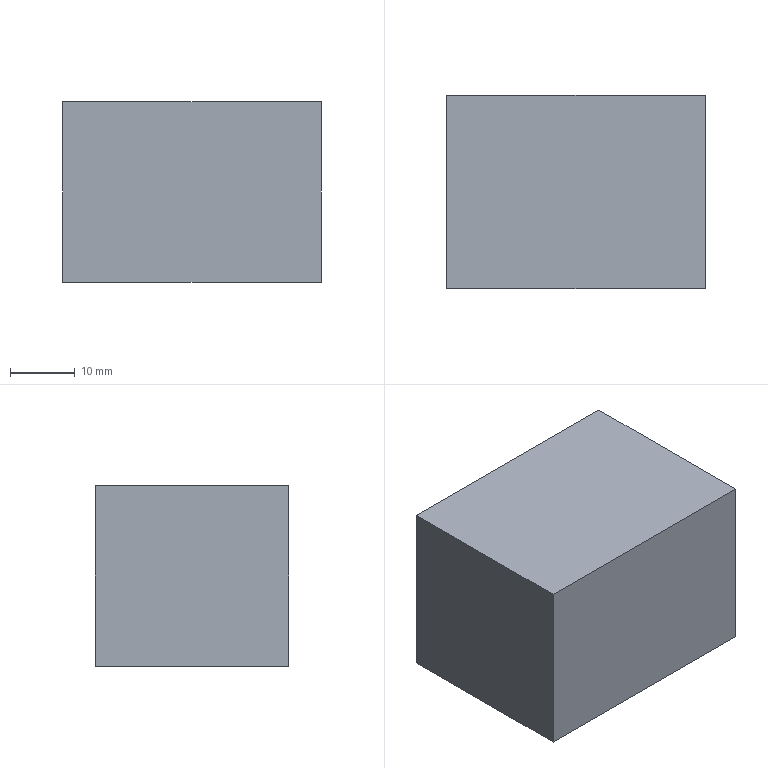Part | NX | features solid 2 | 1 solid | 6 faces | box 40 x 30 x 28 mm | volume 33600 mm3 | plane 6
STEP:
#1=CARTESIAN_POINT('',(-212.,-170.,23.));
#2=VERTEX_POINT('',#1);
#3=CARTESIAN_POINT('',(-252.,-170.,23.));
#4=VERTEX_POINT('',#3);
#5=CARTESIAN_POINT('',(-212.,-170.,23.));
#6=DIRECTION('',(-1.,0.,0.));
#7=VECTOR('',#6,1000.);
#8=LINE('',#5,#7);
#9=EDGE_CURVE('',#2,#4,#8,.T.);
#10=ORIENTED_EDGE('',*,*,#9,.F.);
#11=CARTESIAN_POINT('',(-212.,-140.,23.));
#12=VERTEX_POINT('',#11);
#13=CARTESIAN_POINT('',(-212.,-140.,23.));
#14=DIRECTION('',(0.,-1.,0.));
#15=VECTOR('',#14,1000.);
#16=LINE('',#13,#15);
#17=EDGE_CURVE('',#12,#2,#16,.T.);
#18=ORIENTED_EDGE('',*,*,#17,.F.);
#19=CARTESIAN_POINT('',(-252.,-140.,23.));
#20=VERTEX_POINT('',#19);
#21=CARTESIAN_POINT('',(-212.,-140.,23.));
#22=DIRECTION('',(1.,0.,0.));
#23=VECTOR('',#22,1000.);
#24=LINE('',#21,#23);
#25=EDGE_CURVE('',#12,#20,#24,.F.);
#26=ORIENTED_EDGE('',*,*,#25,.T.);
#27=CARTESIAN_POINT('',(-252.,-140.,23.));
#28=DIRECTION('',(0.,-1.,0.));
#29=VECTOR('',#28,1000.);
#30=LINE('',#27,#29);
#31=EDGE_CURVE('',#20,#4,#30,.T.);
#32=ORIENTED_EDGE('',*,*,#31,.T.);
#33=EDGE_LOOP('',(#10,#18,#26,#32));
#34=FACE_BOUND('',#33,.T.);
#35=CARTESIAN_POINT('',(-212.,-140.,23.));
#36=DIRECTION('',(0.,0.,1.));
#37=DIRECTION('',(0.,-1.,0.));
#38=AXIS2_PLACEMENT_3D('',#35,#36,#37);
#39=PLANE('',#38);
#40=ADVANCED_FACE('',(#34),#39,.T.);
#41=ORIENTED_EDGE('',*,*,#25,.F.);
#42=CARTESIAN_POINT('',(-212.,-140.,-5.));
#43=VERTEX_POINT('',#42);
#44=CARTESIAN_POINT('',(-212.,-140.,85.));
#45=DIRECTION('',(0.,0.,-1.));
#46=VECTOR('',#45,1000.);
#47=LINE('',#44,#46);
#48=EDGE_CURVE('',#12,#43,#47,.T.);
#49=ORIENTED_EDGE('',*,*,#48,.T.);
#50=CARTESIAN_POINT('',(-252.,-140.,-5.));
#51=VERTEX_POINT('',#50);
#52=CARTESIAN_POINT('',(-212.,-140.,-5.));
#53=DIRECTION('',(1.,0.,0.));
#54=VECTOR('',#53,1000.);
#55=LINE('',#52,#54);
#56=EDGE_CURVE('',#43,#51,#55,.F.);
#57=ORIENTED_EDGE('',*,*,#56,.T.);
#58=CARTESIAN_POINT('',(-252.,-140.,85.));
#59=DIRECTION('',(0.,0.,-1.));
#60=VECTOR('',#59,1000.);
#61=LINE('',#58,#60);
#62=EDGE_CURVE('',#20,#51,#61,.T.);
#63=ORIENTED_EDGE('',*,*,#62,.F.);
#64=EDGE_LOOP('',(#41,#49,#57,#63));
#65=FACE_BOUND('',#64,.T.);
#66=CARTESIAN_POINT('',(-212.,-140.,85.));
#67=DIRECTION('',(0.,-1.,0.));
#68=DIRECTION('',(0.,0.,-1.));
#69=AXIS2_PLACEMENT_3D('',#66,#67,#68);
#70=PLANE('',#69);
#71=ADVANCED_FACE('',(#65),#70,.F.);
#72=ORIENTED_EDGE('',*,*,#56,.F.);
#73=CARTESIAN_POINT('',(-212.,-170.,-5.));
#74=VERTEX_POINT('',#73);
#75=CARTESIAN_POINT('',(-212.,-140.,-5.));
#76=DIRECTION('',(0.,-1.,0.));
#77=VECTOR('',#76,1000.);
#78=LINE('',#75,#77);
#79=EDGE_CURVE('',#43,#74,#78,.T.);
#80=ORIENTED_EDGE('',*,*,#79,.T.);
#81=CARTESIAN_POINT('',(-252.,-170.,-5.));
#82=VERTEX_POINT('',#81);
#83=CARTESIAN_POINT('',(-374.173,-170.,-5.));
#84=DIRECTION('',(-1.,0.,0.));
#85=VECTOR('',#84,1000.);
#86=LINE('',#83,#85);
#87=EDGE_CURVE('',#74,#82,#86,.T.);
#88=ORIENTED_EDGE('',*,*,#87,.T.);
#89=CARTESIAN_POINT('',(-252.,-140.,-5.));
#90=DIRECTION('',(0.,-1.,0.));
#91=VECTOR('',#90,1000.);
#92=LINE('',#89,#91);
#93=EDGE_CURVE('',#51,#82,#92,.T.);
#94=ORIENTED_EDGE('',*,*,#93,.F.);
#95=EDGE_LOOP('',(#72,#80,#88,#94));
#96=FACE_BOUND('',#95,.T.);
#97=CARTESIAN_POINT('',(-374.173,-140.,-5.));
#98=DIRECTION('',(0.,0.,-1.));
#99=DIRECTION('',(1.,0.,0.));
#100=AXIS2_PLACEMENT_3D('',#97,#98,#99);
#101=PLANE('',#100);
#102=ADVANCED_FACE('',(#96),#101,.T.);
#103=ORIENTED_EDGE('',*,*,#93,.T.);
#104=CARTESIAN_POINT('',(-252.,-170.,85.));
#105=DIRECTION('',(0.,0.,-1.));
#106=VECTOR('',#105,1000.);
#107=LINE('',#104,#106);
#108=EDGE_CURVE('',#4,#82,#107,.T.);
#109=ORIENTED_EDGE('',*,*,#108,.F.);
#110=ORIENTED_EDGE('',*,*,#31,.F.);
#111=ORIENTED_EDGE('',*,*,#62,.T.);
#112=EDGE_LOOP('',(#103,#109,#110,#111));
#113=FACE_BOUND('',#112,.T.);
#114=CARTESIAN_POINT('',(-252.,-140.,85.));
#115=DIRECTION('',(1.,0.,0.));
#116=DIRECTION('',(0.,0.,-1.));
#117=AXIS2_PLACEMENT_3D('',#114,#115,#116);
#118=PLANE('',#117);
#119=ADVANCED_FACE('',(#113),#118,.F.);
#120=CARTESIAN_POINT('',(-212.,-170.,85.));
#121=DIRECTION('',(0.,0.,-1.));
#122=VECTOR('',#121,1000.);
#123=LINE('',#120,#122);
#124=EDGE_CURVE('',#2,#74,#123,.T.);
#125=ORIENTED_EDGE('',*,*,#124,.F.);
#126=ORIENTED_EDGE('',*,*,#9,.T.);
#127=ORIENTED_EDGE('',*,*,#108,.T.);
#128=ORIENTED_EDGE('',*,*,#87,.F.);
#129=EDGE_LOOP('',(#125,#126,#127,#128));
#130=FACE_BOUND('',#129,.T.);
#131=CARTESIAN_POINT('',(-212.,-170.,85.));
#132=DIRECTION('',(0.,-1.,0.));
#133=DIRECTION('',(0.,0.,-1.));
#134=AXIS2_PLACEMENT_3D('',#131,#132,#133);
#135=PLANE('',#134);
#136=ADVANCED_FACE('',(#130),#135,.T.);
#137=ORIENTED_EDGE('',*,*,#79,.F.);
#138=ORIENTED_EDGE('',*,*,#48,.F.);
#139=ORIENTED_EDGE('',*,*,#17,.T.);
#140=ORIENTED_EDGE('',*,*,#124,.T.);
#141=EDGE_LOOP('',(#137,#138,#139,#140));
#142=FACE_BOUND('',#141,.T.);
#143=CARTESIAN_POINT('',(-212.,-140.,85.));
#144=DIRECTION('',(1.,0.,0.));
#145=DIRECTION('',(0.,0.,-1.));
#146=AXIS2_PLACEMENT_3D('',#143,#144,#145);
#147=PLANE('',#146);
#148=ADVANCED_FACE('',(#142),#147,.T.);
#149=CLOSED_SHELL('',(#40,#71,#102,#119,#136,#148));
#150=MANIFOLD_SOLID_BREP('',#149);
#151=(LENGTH_UNIT()NAMED_UNIT(*)SI_UNIT(.MILLI.,.METRE.));
#152=UNCERTAINTY_MEASURE_WITH_UNIT(LENGTH_MEASURE(0.00001),#151,'','');
#153=(NAMED_UNIT(*)PLANE_ANGLE_UNIT()SI_UNIT($,.RADIAN.));
#154=(NAMED_UNIT(*)SI_UNIT($,.STERADIAN.)SOLID_ANGLE_UNIT());
#155=(GEOMETRIC_REPRESENTATION_CONTEXT(3)GLOBAL_UNCERTAINTY_ASSIGNED_CONTEXT((#152))GLOBAL_UNIT_ASSIGNED_CONTEXT((#151,#153,#154))REPRESENTATION_CONTEXT('',''));
#156=ADVANCED_BREP_SHAPE_REPRESENTATION('',(#150),#155);